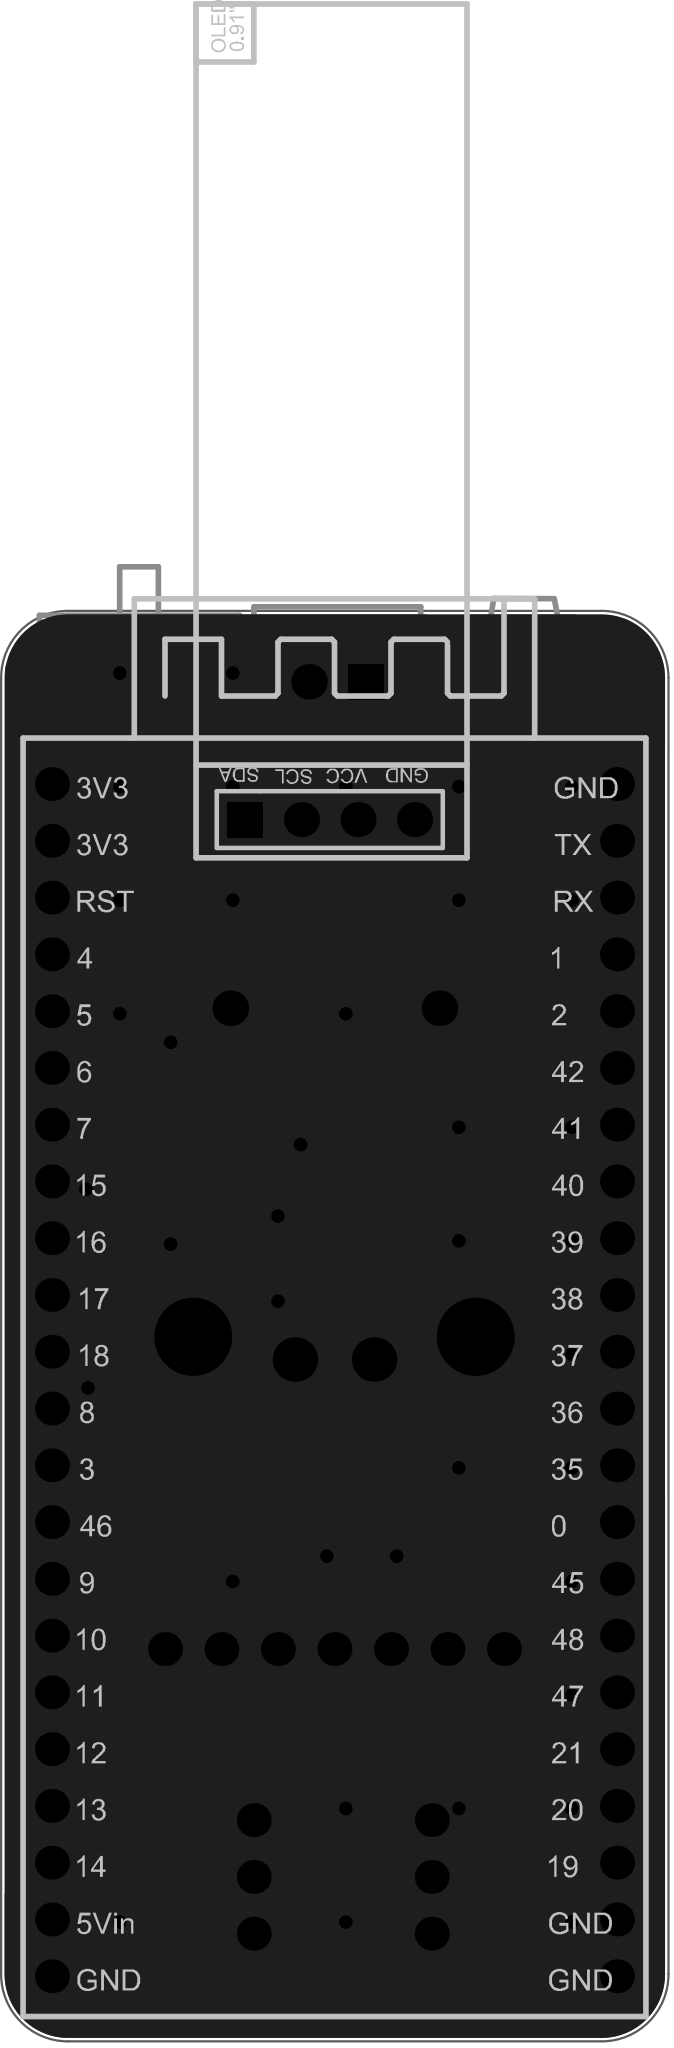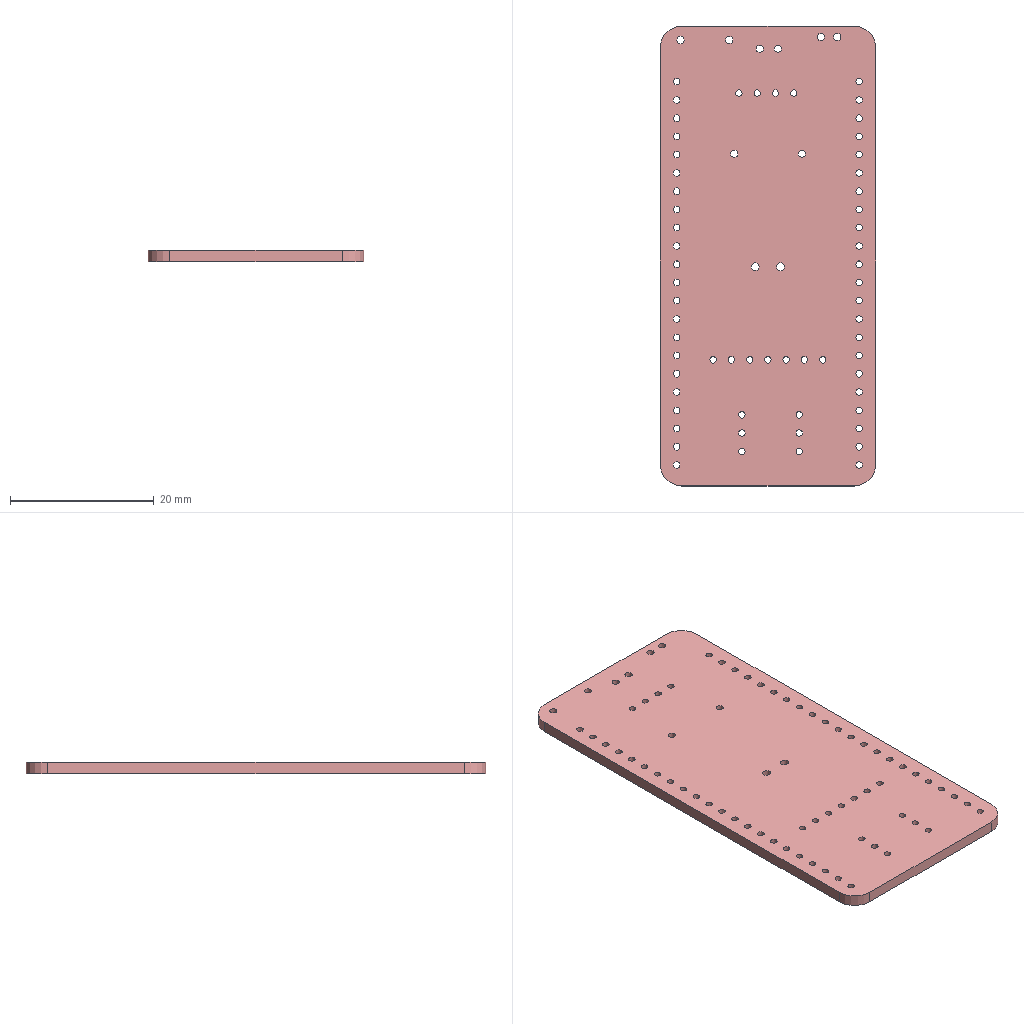Circuit board layout | Altium Designer | box 30 x 64 x 1.6 mm
Layer stack:
# Altium Designer layer stack of  (unit mm; dielectric type: 0 none, 1 core, 2 prepreg, 3 surface material)
index,name,kind,layer,copper_thickness_mm,dielectric_type,dielectric_thickness_mm,dielectric_material,dielectric_constant
0,Top Paste Mask Layer,other,,,,,,
1,Top Silkscreen Layer,other,,,,,,
2,Top Solder Mask Layer,dielectric,,,3,0.01,,3.3
3,Top Layer,copper,Top Layer,0.035,,,,
4,Dielectric1,dielectric,,,3,1.51,FR4,4.5
5,Bottom Layer,copper,Bottom Layer,0.035,,,,
6,Bottom Solder Mask Layer,dielectric,,,3,0.01,,3.3
7,Bottom Silkscreen Layer,other,,,,,,
8,Bottom Paste Mask Layer,other,,,,,,
# drill layer pairs: low layer,high layer
drill_pair,Top Layer,Bottom Layer
Part placement:
Designator,Comment,Layer,Footprint,Center-X(mm),Center-Y(mm),Rotation
OLED1,OLED0.91or0.96,TopLayer,OLED0.91,94.529,132.393,90
U3,Adafruit MAX98357 I2S Amp,BottomLayer,MAX98357_I2S_AMP_MODULE,94.742,101.76,90
U4,NO,TopLayer,ESP32S3,94.742,107.315,0
U9,INMP441,BottomLayer,INMP441,95.115,85.09,180
U11,_x001F_XH2.54-2P,BottomLayer,CONN-TH_2P-P2.54-V,94.869,138.557,180
SPK2,FS-2308,BottomLayer,BEEP-TH_BD23.2-P9.20-D1.0,94.76,123.952,180
U10,GT-TC054A-H038-L1,BottomLayer,SW-SMD_L7.8-W3.5-P4.20-EH,103.251,139.827,180
SW1,SSSS211603,BottomLayer,SW-SMD_SSSS211603,85.979,137.033,180
Pad and via stacks:
# Altium Designer via and pad stacks of  (unit mm). Each distinct definition once, with the count of objects using it.
# via: kind,start_layer,end_layer,hole_mm,diameter_mm,mode(0 simple;1 top-mid-bottom;2 full stack),diameter_per_layer,count,example_net
# pad: kind,layer,hole_mm,hole_type(0 round;1 square;2 slot),plating,top_size,top_shape(1 round;2 rect;3 octagon;9 rounded rect),mid_size,bottom_size,mode,footprint,size_per_layer,count,example
pad,Multi-Layer,0.889,0,plated,1.575x1.575,1,1.575x1.575,1.575x1.575,0,OLED0.91,,3,OLED1.4
pad,Multi-Layer,0.889,0,plated,1.575x1.575,2,1.575x1.575,1.575x1.575,0,OLED0.91,,1,OLED1.1
pad,Multi-Layer,0.9144,0,plated,1.524x1.524,1,1.524x1.524,1.524x1.524,0,MAX98357 I2S AMP MODULE,,7,U3.1
pad,Multi-Layer,1.1,0,plated,2x2,1,2x2,2x2,0,MAX98357 I2S AMP MODULE,,2,U3.9
pad,Multi-Layer,0.9144,0,plated,1.524x1.524,1,1.524x1.524,1.524x1.524,0,ESP32S3,,44,U4.1
pad,Multi-Layer,0.9144,0,plated,1.524x1.524,1,1.524x1.524,1.524x1.524,0,INMP441,,6,U9.5
pad,Multi-Layer,1,0,plated,1.6x1.6,1,1.6x1.6,1.6x1.6,0,CONN-TH_2P-P2.54-V,,1,U11.2
pad,Multi-Layer,1,0,plated,1.6x1.6,2,1.6x1.6,1.6x1.6,0,CONN-TH_2P-P2.54-V,,1,U11.1
pad,Multi-Layer,1,0,plated,1.6x1.6,1,1.6x1.6,1.6x1.6,0,BEEP-TH_BD23.2-P9.20-D1.0,,2,SPK2.1
pad,Bottom Layer,0,0,plated,1.5x1.5,2,1.5x1.5,1.5x1.5,0,SW-SMD_L7.8-W3.5-P4.20-EH,,2,U10.4
pad,Bottom Layer,0,0,plated,0.9x1.2,2,0.9x1.2,0.9x1.2,0,SW-SMD_L7.8-W3.5-P4.20-EH,,2,U10.2
pad,Bottom Layer,0,0,plated,1.2x2.5,2,1.2x2.5,1.2x2.5,0,SW-SMD_SSSS211603,,3,SW1.1
via,Top Layer,Bottom Layer,0.3048,0.6096,0,,33,16
via,Top Layer,Bottom Layer,0.3048,0.61,0,,5,GND
via,Top Layer,Bottom Layer,2.499,3.5,0,,2,
Copper pours:
name,layer,net,type(0 solid;1 hatched;2 none)
Bottom Layer-GND,Bottom Layer,GND,0
Top Layer-GND,Top Layer,GND,0
Design rules, without the lines most boards share:
# Altium Designer design rules of  (exported by Altium Designer, unit mm)
# columns: name | kind | enabled | priority | scope1 | scope2 | descriptor | typed fields (field=value)
Plane_Default | 0 | disabled | 1 | All | All | Clearance Constraint (Gap=6mil) (Disabled)(All),(All) | gap=0.1524
Plane_Default_1 | 63 | disabled | 1 | All | All | Board Clearance Constraint (Gap=0mil) (Disabled)(All) |
Copper_Default | 0 | disabled | 2 | All | All | Clearance Constraint (Gap=6mil) (Disabled)(All),(All) | gap=0.1524
Copper_Default_1 | 63 | disabled | 2 | All | All | Board Clearance Constraint (Gap=0mil) (Disabled)(All) |
Copper_gge24019 | 0 | disabled | 3 | All | All | Clearance Constraint (Gap=6mil) (Disabled)(All),(All) | gap=0.1524
Copper_gge24019_1 | 63 | disabled | 3 | All | All | Board Clearance Constraint (Gap=0mil) (Disabled)(All) |
Default | 0 | enabled | 4 | All | All | Clearance Constraint (Gap=6mil) (All),(All) | gap=0.1524
Default_1 | 63 | enabled | 4 | All | All | Board Clearance Constraint (Gap=0mil) (All) |
otherClearance | 52 | enabled | 1 | All | All | Hole To Hole Clearance (Gap=11.8mil) (All),(All) | gap=0.2997
Default_2 | 2 | enabled | 1 | All | All | Width Constraint (Min=10mil) (Max=1000mil) (Preferred=30mil) (All) |
Default_3 | 11 | enabled | 1 | All | All | Routing Via (MinHoleWidth=12mil) (MaxHoleWidth=2362mil) (PreferredHoleWidth=12mil) (MinWidth=24mil) (MaxWidth=3938mil) (PreferedWidth=24mil) (All) | via_min_hole=0.3048 via_max_hole=59.995 via_preferred_diameter=0.6096 via_preferred_hole=0.3048
Default_4 | 6 | enabled | 1 | All | All | Power Plane Connect Rule(Relief Connect )(Expansion=20mil) (Conductor Width=0mil) (Air Gap=10mil) (Entries=4) (All) | relief_conductor_width=0 relief_entries=4 relief_expansion=0.508
gge24019 | 20 | disabled | 1 | All | All | Polygon Connect Rule(Relief Connect )(Conductor Width=0mil) (Relief Angle=90 Angle) (Entries=4) (Air Gap Width=1mil) (Disabled)(All),(All) | connect_style(0=relief,1=direct,2=none)=0 relief_conductor_width=0 relief_entries=4
Default_5 | 20 | enabled | 2 | All | All | Polygon Connect Rule(Relief Connect )(Conductor Width=0mil) (Relief Angle=90 Angle) (Entries=4) (Air Gap Width=1mil) (All),(All) | connect_style(0=relief,1=direct,2=none)=0 relief_conductor_width=0 relief_entries=4
Common | 14 | enabled | 1 | All | All | Paste Mask Expansion (Expansion =0mil) (All) | expansion=0
Common_1 | 13 | enabled | 2 | All | All | Solder Mask Expansion (Expansion =2mil) (All) | expansion=0.0508
Common_2 | 13 | enabled | 1 | IsVia | All | Solder Mask Expansion (Expansion =-1000mil) (IsVia) | expansion=-25.4